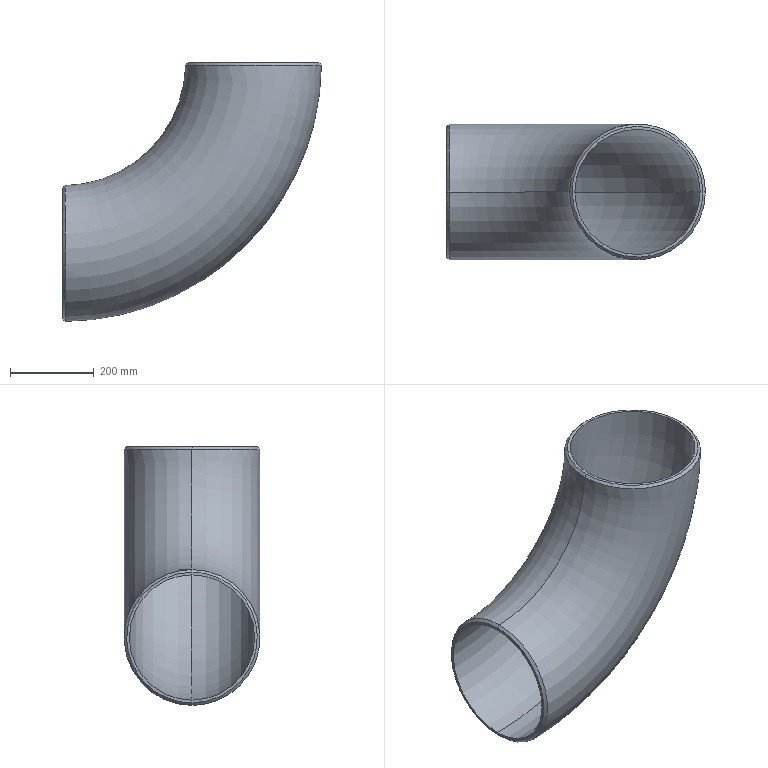Part | NX | features BREP 1 | 1 solid | 10 faces | box 619.473 x 325 x 619.47 mm | volume 8769531 mm3 | spline 4 | torus 4 | plane 2